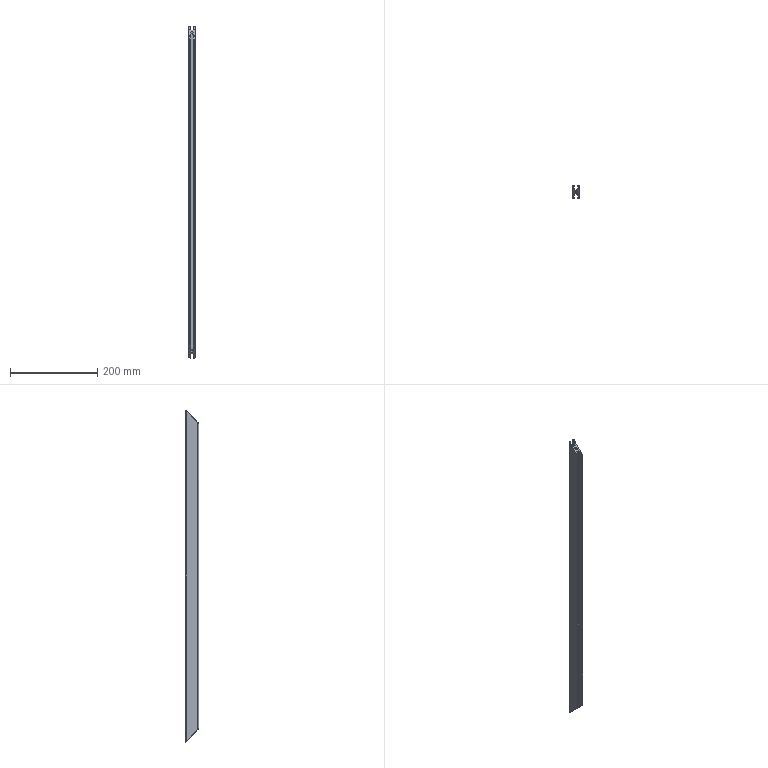Part | STEP file | OB1530-760 | 1 solid | 36 faces | box 15 x 30 x 760 mm | volume 178437 mm3 | plane 30 | cylinder 6 | commonest cylinder face diameters 3 x4 5 x2
STEP:
#1=CARTESIAN_POINT('',(2.5,0.,745.));
#2=VERTEX_POINT('',#1);
#3=CARTESIAN_POINT('',(-2.5,0.,745.));
#4=VERTEX_POINT('',#3);
#5=CARTESIAN_POINT('',(2.5,0.,745.));
#6=CARTESIAN_POINT('',(2.5,-5.,740.));
#7=CARTESIAN_POINT('',(-2.5,-5.,740.));
#8=CARTESIAN_POINT('',(-2.5,0.,745.));
#9=(BOUNDED_CURVE()B_SPLINE_CURVE(3,(#5,#6,#7,#8),.UNSPECIFIED.,.F.,.F.)B_SPLINE_CURVE_WITH_KNOTS((4,4),(4.712,7.854),.UNSPECIFIED.)CURVE()GEOMETRIC_REPRESENTATION_ITEM()RATIONAL_B_SPLINE_CURVE((1.,0.3333,0.3333,1.))REPRESENTATION_ITEM(''));
#10=EDGE_CURVE('',#2,#4,#9,.T.);
#11=ORIENTED_EDGE('',*,*,#10,.F.);
#12=CARTESIAN_POINT('',(2.5,0.,15.));
#13=VERTEX_POINT('',#12);
#14=CARTESIAN_POINT('',(2.5,0.,760.));
#15=DIRECTION('',(0.,0.,-1.));
#16=VECTOR('',#15,1000.);
#17=LINE('',#14,#16);
#18=EDGE_CURVE('',#2,#13,#17,.T.);
#19=ORIENTED_EDGE('',*,*,#18,.T.);
#20=CARTESIAN_POINT('',(-2.5,0.,15.));
#21=VERTEX_POINT('',#20);
#22=CARTESIAN_POINT('',(-2.5,0.,15.));
#23=CARTESIAN_POINT('',(-2.5,-5.,20.));
#24=CARTESIAN_POINT('',(2.5,-5.,20.));
#25=CARTESIAN_POINT('',(2.5,0.,15.));
#26=(BOUNDED_CURVE()B_SPLINE_CURVE(3,(#22,#23,#24,#25),.UNSPECIFIED.,.F.,.F.)B_SPLINE_CURVE_WITH_KNOTS((4,4),(1.571,4.712),.UNSPECIFIED.)CURVE()GEOMETRIC_REPRESENTATION_ITEM()RATIONAL_B_SPLINE_CURVE((1.,0.3333,0.3333,1.))REPRESENTATION_ITEM(''));
#27=EDGE_CURVE('',#21,#13,#26,.T.);
#28=ORIENTED_EDGE('',*,*,#27,.F.);
#29=CARTESIAN_POINT('',(-2.5,0.,760.));
#30=DIRECTION('',(0.,0.,-1.));
#31=VECTOR('',#30,1000.);
#32=LINE('',#29,#31);
#33=EDGE_CURVE('',#4,#21,#32,.T.);
#34=ORIENTED_EDGE('',*,*,#33,.F.);
#35=EDGE_LOOP('',(#11,#19,#28,#34));
#36=FACE_OUTER_BOUND('',#35,.T.);
#37=CARTESIAN_POINT('',(0.,0.,760.));
#38=DIRECTION('',(0.,0.,-1.));
#39=DIRECTION('',(-1.,0.,0.));
#40=AXIS2_PLACEMENT_3D('',#37,#38,#39);
#41=CYLINDRICAL_SURFACE('',#40,2.5);
#42=ADVANCED_FACE('',(#36),#41,.F.);
#43=CARTESIAN_POINT('',(6.,15.,760.));
#44=VERTEX_POINT('',#43);
#45=CARTESIAN_POINT('',(6.,15.,0.));
#46=VERTEX_POINT('',#45);
#47=CARTESIAN_POINT('',(6.,15.,760.));
#48=DIRECTION('',(0.,0.,-1.));
#49=VECTOR('',#48,1000.);
#50=LINE('',#47,#49);
#51=EDGE_CURVE('',#44,#46,#50,.T.);
#52=ORIENTED_EDGE('',*,*,#51,.F.);
#53=CARTESIAN_POINT('',(7.5,13.5,758.5));
#54=VERTEX_POINT('',#53);
#55=CARTESIAN_POINT('',(6.,15.,760.));
#56=CARTESIAN_POINT('',(6.879,15.,760.));
#57=CARTESIAN_POINT('',(7.5,14.379,759.379));
#58=CARTESIAN_POINT('',(7.5,13.5,758.5));
#59=(BOUNDED_CURVE()B_SPLINE_CURVE(3,(#55,#56,#57,#58),.UNSPECIFIED.,.F.,.T.)B_SPLINE_CURVE_WITH_KNOTS((4,4),(3.142,4.712),.UNSPECIFIED.)CURVE()GEOMETRIC_REPRESENTATION_ITEM()RATIONAL_B_SPLINE_CURVE((1.,0.8047,0.8047,1.))REPRESENTATION_ITEM(''));
#60=EDGE_CURVE('',#44,#54,#59,.T.);
#61=ORIENTED_EDGE('',*,*,#60,.T.);
#62=CARTESIAN_POINT('',(7.5,13.5,1.5));
#63=VERTEX_POINT('',#62);
#64=CARTESIAN_POINT('',(7.5,13.5,760.));
#65=DIRECTION('',(0.,0.,-1.));
#66=VECTOR('',#65,1000.);
#67=LINE('',#64,#66);
#68=EDGE_CURVE('',#54,#63,#67,.T.);
#69=ORIENTED_EDGE('',*,*,#68,.T.);
#70=CARTESIAN_POINT('',(7.5,13.5,1.5));
#71=CARTESIAN_POINT('',(7.5,14.379,0.6213));
#72=CARTESIAN_POINT('',(6.879,15.,0.));
#73=CARTESIAN_POINT('',(6.,15.,0.));
#74=(BOUNDED_CURVE()B_SPLINE_CURVE(3,(#70,#71,#72,#73),.UNSPECIFIED.,.F.,.F.)B_SPLINE_CURVE_WITH_KNOTS((4,4),(4.712,6.283),.UNSPECIFIED.)CURVE()GEOMETRIC_REPRESENTATION_ITEM()RATIONAL_B_SPLINE_CURVE((1.,0.8047,0.8047,1.))REPRESENTATION_ITEM(''));
#75=EDGE_CURVE('',#63,#46,#74,.T.);
#76=ORIENTED_EDGE('',*,*,#75,.T.);
#77=EDGE_LOOP('',(#52,#61,#69,#76));
#78=FACE_OUTER_BOUND('',#77,.T.);
#79=CARTESIAN_POINT('',(6.,13.5,760.));
#80=DIRECTION('',(0.,0.,-1.));
#81=DIRECTION('',(-1.,0.,0.));
#82=AXIS2_PLACEMENT_3D('',#79,#80,#81);
#83=CYLINDRICAL_SURFACE('',#82,1.5);
#84=ADVANCED_FACE('',(#78),#83,.T.);
#85=CARTESIAN_POINT('',(3.25,15.,0.));
#86=VERTEX_POINT('',#85);
#87=CARTESIAN_POINT('',(6.,15.,0.));
#88=DIRECTION('',(-1.,0.,0.));
#89=VECTOR('',#88,1000.);
#90=LINE('',#87,#89);
#91=EDGE_CURVE('',#46,#86,#90,.T.);
#92=ORIENTED_EDGE('',*,*,#91,.T.);
#93=CARTESIAN_POINT('',(3.25,15.,760.));
#94=VERTEX_POINT('',#93);
#95=CARTESIAN_POINT('',(3.25,15.,760.));
#96=DIRECTION('',(0.,0.,-1.));
#97=VECTOR('',#96,1000.);
#98=LINE('',#95,#97);
#99=EDGE_CURVE('',#94,#86,#98,.T.);
#100=ORIENTED_EDGE('',*,*,#99,.F.);
#101=CARTESIAN_POINT('',(6.,15.,760.));
#102=DIRECTION('',(-1.,0.,0.));
#103=VECTOR('',#102,1000.);
#104=LINE('',#101,#103);
#105=EDGE_CURVE('',#44,#94,#104,.T.);
#106=ORIENTED_EDGE('',*,*,#105,.F.);
#107=ORIENTED_EDGE('',*,*,#51,.T.);
#108=EDGE_LOOP('',(#92,#100,#106,#107));
#109=FACE_OUTER_BOUND('',#108,.T.);
#110=CARTESIAN_POINT('',(6.,15.,760.));
#111=DIRECTION('',(0.,-1.,0.));
#112=DIRECTION('',(0.,0.,-1.));
#113=AXIS2_PLACEMENT_3D('',#110,#111,#112);
#114=PLANE('',#113);
#115=ADVANCED_FACE('',(#109),#114,.F.);
#116=CARTESIAN_POINT('',(3.25,13.,758.));
#117=VERTEX_POINT('',#116);
#118=CARTESIAN_POINT('',(3.25,13.,2.));
#119=VERTEX_POINT('',#118);
#120=CARTESIAN_POINT('',(3.25,13.,760.));
#121=DIRECTION('',(0.,0.,-1.));
#122=VECTOR('',#121,1000.);
#123=LINE('',#120,#122);
#124=EDGE_CURVE('',#117,#119,#123,.T.);
#125=ORIENTED_EDGE('',*,*,#124,.F.);
#126=CARTESIAN_POINT('',(3.25,15.,760.));
#127=DIRECTION('',(0.,0.7071,0.7071));
#128=VECTOR('',#127,1000.);
#129=LINE('',#126,#128);
#130=EDGE_CURVE('',#117,#94,#129,.T.);
#131=ORIENTED_EDGE('',*,*,#130,.T.);
#132=ORIENTED_EDGE('',*,*,#99,.T.);
#133=CARTESIAN_POINT('',(3.25,-365.,380.));
#134=DIRECTION('',(0.,-0.7071,0.7071));
#135=VECTOR('',#134,1000.);
#136=LINE('',#133,#135);
#137=EDGE_CURVE('',#86,#119,#136,.T.);
#138=ORIENTED_EDGE('',*,*,#137,.T.);
#139=EDGE_LOOP('',(#125,#131,#132,#138));
#140=FACE_OUTER_BOUND('',#139,.T.);
#141=CARTESIAN_POINT('',(3.25,15.,760.));
#142=DIRECTION('',(1.,0.,0.));
#143=DIRECTION('',(0.,0.,-1.));
#144=AXIS2_PLACEMENT_3D('',#141,#142,#143);
#145=PLANE('',#144);
#146=ADVANCED_FACE('',(#140),#145,.F.);
#147=CARTESIAN_POINT('',(5.5,13.,758.));
#148=VERTEX_POINT('',#147);
#149=CARTESIAN_POINT('',(5.5,13.,2.));
#150=VERTEX_POINT('',#149);
#151=CARTESIAN_POINT('',(5.5,13.,760.));
#152=DIRECTION('',(0.,0.,-1.));
#153=VECTOR('',#152,1000.);
#154=LINE('',#151,#153);
#155=EDGE_CURVE('',#148,#150,#154,.T.);
#156=ORIENTED_EDGE('',*,*,#155,.F.);
#157=CARTESIAN_POINT('',(3.25,13.,758.));
#158=DIRECTION('',(-1.,0.,0.));
#159=VECTOR('',#158,1000.);
#160=LINE('',#157,#159);
#161=EDGE_CURVE('',#148,#117,#160,.T.);
#162=ORIENTED_EDGE('',*,*,#161,.T.);
#163=ORIENTED_EDGE('',*,*,#124,.T.);
#164=CARTESIAN_POINT('',(3.25,13.,2.));
#165=DIRECTION('',(1.,0.,0.));
#166=VECTOR('',#165,1000.);
#167=LINE('',#164,#166);
#168=EDGE_CURVE('',#119,#150,#167,.T.);
#169=ORIENTED_EDGE('',*,*,#168,.T.);
#170=EDGE_LOOP('',(#156,#162,#163,#169));
#171=FACE_OUTER_BOUND('',#170,.T.);
#172=CARTESIAN_POINT('',(3.25,13.,760.));
#173=DIRECTION('',(0.,1.,0.));
#174=DIRECTION('',(0.,0.,1.));
#175=AXIS2_PLACEMENT_3D('',#172,#173,#174);
#176=PLANE('',#175);
#177=ADVANCED_FACE('',(#171),#176,.F.);
#178=CARTESIAN_POINT('',(5.5,7.,752.));
#179=VERTEX_POINT('',#178);
#180=CARTESIAN_POINT('',(5.5,7.,8.));
#181=VERTEX_POINT('',#180);
#182=CARTESIAN_POINT('',(5.5,7.,760.));
#183=DIRECTION('',(0.,0.,-1.));
#184=VECTOR('',#183,1000.);
#185=LINE('',#182,#184);
#186=EDGE_CURVE('',#179,#181,#185,.T.);
#187=ORIENTED_EDGE('',*,*,#186,.F.);
#188=CARTESIAN_POINT('',(5.5,14.,759.));
#189=DIRECTION('',(0.,0.7071,0.7071));
#190=VECTOR('',#189,1000.);
#191=LINE('',#188,#190);
#192=EDGE_CURVE('',#179,#148,#191,.T.);
#193=ORIENTED_EDGE('',*,*,#192,.T.);
#194=ORIENTED_EDGE('',*,*,#155,.T.);
#195=CARTESIAN_POINT('',(5.5,-366.,381.));
#196=DIRECTION('',(0.,-0.7071,0.7071));
#197=VECTOR('',#196,1000.);
#198=LINE('',#195,#197);
#199=EDGE_CURVE('',#150,#181,#198,.T.);
#200=ORIENTED_EDGE('',*,*,#199,.T.);
#201=EDGE_LOOP('',(#187,#193,#194,#200));
#202=FACE_OUTER_BOUND('',#201,.T.);
#203=CARTESIAN_POINT('',(5.5,13.,760.));
#204=DIRECTION('',(1.,0.,0.));
#205=DIRECTION('',(0.,1.,0.));
#206=AXIS2_PLACEMENT_3D('',#203,#204,#205);
#207=PLANE('',#206);
#208=ADVANCED_FACE('',(#202),#207,.F.);
#209=CARTESIAN_POINT('',(3.25,7.,752.));
#210=VERTEX_POINT('',#209);
#211=CARTESIAN_POINT('',(3.25,7.,8.));
#212=VERTEX_POINT('',#211);
#213=CARTESIAN_POINT('',(3.25,7.,760.));
#214=DIRECTION('',(0.,0.,-1.));
#215=VECTOR('',#214,1000.);
#216=LINE('',#213,#215);
#217=EDGE_CURVE('',#210,#212,#216,.T.);
#218=ORIENTED_EDGE('',*,*,#217,.F.);
#219=CARTESIAN_POINT('',(5.5,7.,752.));
#220=DIRECTION('',(1.,0.,0.));
#221=VECTOR('',#220,1000.);
#222=LINE('',#219,#221);
#223=EDGE_CURVE('',#210,#179,#222,.T.);
#224=ORIENTED_EDGE('',*,*,#223,.T.);
#225=ORIENTED_EDGE('',*,*,#186,.T.);
#226=CARTESIAN_POINT('',(5.5,7.,8.));
#227=DIRECTION('',(-1.,0.,0.));
#228=VECTOR('',#227,1000.);
#229=LINE('',#226,#228);
#230=EDGE_CURVE('',#181,#212,#229,.T.);
#231=ORIENTED_EDGE('',*,*,#230,.T.);
#232=EDGE_LOOP('',(#218,#224,#225,#231));
#233=FACE_OUTER_BOUND('',#232,.T.);
#234=CARTESIAN_POINT('',(5.5,7.,760.));
#235=DIRECTION('',(0.,-1.,0.));
#236=DIRECTION('',(1.,0.,0.));
#237=AXIS2_PLACEMENT_3D('',#234,#235,#236);
#238=PLANE('',#237);
#239=ADVANCED_FACE('',(#233),#238,.F.);
#240=CARTESIAN_POINT('',(3.25,5.,750.));
#241=VERTEX_POINT('',#240);
#242=CARTESIAN_POINT('',(3.25,5.,10.));
#243=VERTEX_POINT('',#242);
#244=CARTESIAN_POINT('',(3.25,5.,760.));
#245=DIRECTION('',(0.,0.,-1.));
#246=VECTOR('',#245,1000.);
#247=LINE('',#244,#246);
#248=EDGE_CURVE('',#241,#243,#247,.T.);
#249=ORIENTED_EDGE('',*,*,#248,.F.);
#250=CARTESIAN_POINT('',(3.25,11.,756.));
#251=DIRECTION('',(0.,0.7071,0.7071));
#252=VECTOR('',#251,1000.);
#253=LINE('',#250,#252);
#254=EDGE_CURVE('',#241,#210,#253,.T.);
#255=ORIENTED_EDGE('',*,*,#254,.T.);
#256=ORIENTED_EDGE('',*,*,#217,.T.);
#257=CARTESIAN_POINT('',(3.25,-369.,384.));
#258=DIRECTION('',(0.,-0.7071,0.7071));
#259=VECTOR('',#258,1000.);
#260=LINE('',#257,#259);
#261=EDGE_CURVE('',#212,#243,#260,.T.);
#262=ORIENTED_EDGE('',*,*,#261,.T.);
#263=EDGE_LOOP('',(#249,#255,#256,#262));
#264=FACE_OUTER_BOUND('',#263,.T.);
#265=CARTESIAN_POINT('',(3.25,7.,760.));
#266=DIRECTION('',(1.,0.,0.));
#267=DIRECTION('',(0.,1.,0.));
#268=AXIS2_PLACEMENT_3D('',#265,#266,#267);
#269=PLANE('',#268);
#270=ADVANCED_FACE('',(#264),#269,.F.);
#271=CARTESIAN_POINT('',(-3.25,5.,750.));
#272=VERTEX_POINT('',#271);
#273=CARTESIAN_POINT('',(-3.25,5.,10.));
#274=VERTEX_POINT('',#273);
#275=CARTESIAN_POINT('',(-3.25,5.,760.));
#276=DIRECTION('',(0.,0.,-1.));
#277=VECTOR('',#276,1000.);
#278=LINE('',#275,#277);
#279=EDGE_CURVE('',#272,#274,#278,.T.);
#280=ORIENTED_EDGE('',*,*,#279,.F.);
#281=CARTESIAN_POINT('',(3.25,5.,750.));
#282=DIRECTION('',(1.,0.,0.));
#283=VECTOR('',#282,1000.);
#284=LINE('',#281,#283);
#285=EDGE_CURVE('',#272,#241,#284,.T.);
#286=ORIENTED_EDGE('',*,*,#285,.T.);
#287=ORIENTED_EDGE('',*,*,#248,.T.);
#288=CARTESIAN_POINT('',(3.25,5.,10.));
#289=DIRECTION('',(-1.,0.,0.));
#290=VECTOR('',#289,1000.);
#291=LINE('',#288,#290);
#292=EDGE_CURVE('',#243,#274,#291,.T.);
#293=ORIENTED_EDGE('',*,*,#292,.T.);
#294=EDGE_LOOP('',(#280,#286,#287,#293));
#295=FACE_OUTER_BOUND('',#294,.T.);
#296=CARTESIAN_POINT('',(3.25,5.,760.));
#297=DIRECTION('',(0.,-1.,0.));
#298=DIRECTION('',(0.,0.,-1.));
#299=AXIS2_PLACEMENT_3D('',#296,#297,#298);
#300=PLANE('',#299);
#301=ADVANCED_FACE('',(#295),#300,.F.);
#302=CARTESIAN_POINT('',(-3.25,7.,752.));
#303=VERTEX_POINT('',#302);
#304=CARTESIAN_POINT('',(-3.25,7.,8.));
#305=VERTEX_POINT('',#304);
#306=CARTESIAN_POINT('',(-3.25,7.,760.));
#307=DIRECTION('',(0.,0.,-1.));
#308=VECTOR('',#307,1000.);
#309=LINE('',#306,#308);
#310=EDGE_CURVE('',#303,#305,#309,.T.);
#311=ORIENTED_EDGE('',*,*,#310,.F.);
#312=CARTESIAN_POINT('',(-3.25,11.,756.));
#313=DIRECTION('',(0.,-0.7071,-0.7071));
#314=VECTOR('',#313,1000.);
#315=LINE('',#312,#314);
#316=EDGE_CURVE('',#303,#272,#315,.T.);
#317=ORIENTED_EDGE('',*,*,#316,.T.);
#318=ORIENTED_EDGE('',*,*,#279,.T.);
#319=CARTESIAN_POINT('',(-3.25,-369.,384.));
#320=DIRECTION('',(0.,0.7071,-0.7071));
#321=VECTOR('',#320,1000.);
#322=LINE('',#319,#321);
#323=EDGE_CURVE('',#274,#305,#322,.T.);
#324=ORIENTED_EDGE('',*,*,#323,.T.);
#325=EDGE_LOOP('',(#311,#317,#318,#324));
#326=FACE_OUTER_BOUND('',#325,.T.);
#327=CARTESIAN_POINT('',(-3.25,7.,760.));
#328=DIRECTION('',(-1.,0.,0.));
#329=DIRECTION('',(0.,-1.,0.));
#330=AXIS2_PLACEMENT_3D('',#327,#328,#329);
#331=PLANE('',#330);
#332=ADVANCED_FACE('',(#326),#331,.F.);
#333=CARTESIAN_POINT('',(-5.5,7.,752.));
#334=VERTEX_POINT('',#333);
#335=CARTESIAN_POINT('',(-5.5,7.,8.));
#336=VERTEX_POINT('',#335);
#337=CARTESIAN_POINT('',(-5.5,7.,760.));
#338=DIRECTION('',(0.,0.,-1.));
#339=VECTOR('',#338,1000.);
#340=LINE('',#337,#339);
#341=EDGE_CURVE('',#334,#336,#340,.T.);
#342=ORIENTED_EDGE('',*,*,#341,.F.);
#343=CARTESIAN_POINT('',(-5.5,7.,752.));
#344=DIRECTION('',(1.,0.,0.));
#345=VECTOR('',#344,1000.);
#346=LINE('',#343,#345);
#347=EDGE_CURVE('',#334,#303,#346,.T.);
#348=ORIENTED_EDGE('',*,*,#347,.T.);
#349=ORIENTED_EDGE('',*,*,#310,.T.);
#350=CARTESIAN_POINT('',(-5.5,7.,8.));
#351=DIRECTION('',(-1.,0.,0.));
#352=VECTOR('',#351,1000.);
#353=LINE('',#350,#352);
#354=EDGE_CURVE('',#305,#336,#353,.T.);
#355=ORIENTED_EDGE('',*,*,#354,.T.);
#356=EDGE_LOOP('',(#342,#348,#349,#355));
#357=FACE_OUTER_BOUND('',#356,.T.);
#358=CARTESIAN_POINT('',(-5.5,7.,760.));
#359=DIRECTION('',(0.,-1.,0.));
#360=DIRECTION('',(1.,0.,0.));
#361=AXIS2_PLACEMENT_3D('',#358,#359,#360);
#362=PLANE('',#361);
#363=ADVANCED_FACE('',(#357),#362,.F.);
#364=CARTESIAN_POINT('',(-5.5,13.,758.));
#365=VERTEX_POINT('',#364);
#366=CARTESIAN_POINT('',(-5.5,13.,2.));
#367=VERTEX_POINT('',#366);
#368=CARTESIAN_POINT('',(-5.5,13.,760.));
#369=DIRECTION('',(0.,0.,-1.));
#370=VECTOR('',#369,1000.);
#371=LINE('',#368,#370);
#372=EDGE_CURVE('',#365,#367,#371,.T.);
#373=ORIENTED_EDGE('',*,*,#372,.F.);
#374=CARTESIAN_POINT('',(-5.5,14.,759.));
#375=DIRECTION('',(0.,-0.7071,-0.7071));
#376=VECTOR('',#375,1000.);
#377=LINE('',#374,#376);
#378=EDGE_CURVE('',#365,#334,#377,.T.);
#379=ORIENTED_EDGE('',*,*,#378,.T.);
#380=ORIENTED_EDGE('',*,*,#341,.T.);
#381=CARTESIAN_POINT('',(-5.5,-366.,381.));
#382=DIRECTION('',(0.,0.7071,-0.7071));
#383=VECTOR('',#382,1000.);
#384=LINE('',#381,#383);
#385=EDGE_CURVE('',#336,#367,#384,.T.);
#386=ORIENTED_EDGE('',*,*,#385,.T.);
#387=EDGE_LOOP('',(#373,#379,#380,#386));
#388=FACE_OUTER_BOUND('',#387,.T.);
#389=CARTESIAN_POINT('',(-5.5,13.,760.));
#390=DIRECTION('',(-1.,0.,0.));
#391=DIRECTION('',(0.,-1.,0.));
#392=AXIS2_PLACEMENT_3D('',#389,#390,#391);
#393=PLANE('',#392);
#394=ADVANCED_FACE('',(#388),#393,.F.);
#395=CARTESIAN_POINT('',(-3.25,13.,758.));
#396=VERTEX_POINT('',#395);
#397=CARTESIAN_POINT('',(-3.25,13.,2.));
#398=VERTEX_POINT('',#397);
#399=CARTESIAN_POINT('',(-3.25,13.,760.));
#400=DIRECTION('',(0.,0.,-1.));
#401=VECTOR('',#400,1000.);
#402=LINE('',#399,#401);
#403=EDGE_CURVE('',#396,#398,#402,.T.);
#404=ORIENTED_EDGE('',*,*,#403,.F.);
#405=CARTESIAN_POINT('',(-3.25,13.,758.));
#406=DIRECTION('',(-1.,0.,0.));
#407=VECTOR('',#406,1000.);
#408=LINE('',#405,#407);
#409=EDGE_CURVE('',#396,#365,#408,.T.);
#410=ORIENTED_EDGE('',*,*,#409,.T.);
#411=ORIENTED_EDGE('',*,*,#372,.T.);
#412=CARTESIAN_POINT('',(-3.25,13.,2.));
#413=DIRECTION('',(1.,0.,0.));
#414=VECTOR('',#413,1000.);
#415=LINE('',#412,#414);
#416=EDGE_CURVE('',#367,#398,#415,.T.);
#417=ORIENTED_EDGE('',*,*,#416,.T.);
#418=EDGE_LOOP('',(#404,#410,#411,#417));
#419=FACE_OUTER_BOUND('',#418,.T.);
#420=CARTESIAN_POINT('',(-3.25,13.,760.));
#421=DIRECTION('',(0.,1.,0.));
#422=DIRECTION('',(0.,0.,1.));
#423=AXIS2_PLACEMENT_3D('',#420,#421,#422);
#424=PLANE('',#423);
#425=ADVANCED_FACE('',(#419),#424,.F.);
#426=CARTESIAN_POINT('',(-3.25,15.,760.));
#427=VERTEX_POINT('',#426);
#428=CARTESIAN_POINT('',(-3.25,15.,0.));
#429=VERTEX_POINT('',#428);
#430=CARTESIAN_POINT('',(-3.25,15.,760.));
#431=DIRECTION('',(0.,0.,-1.));
#432=VECTOR('',#431,1000.);
#433=LINE('',#430,#432);
#434=EDGE_CURVE('',#427,#429,#433,.T.);
#435=ORIENTED_EDGE('',*,*,#434,.F.);
#436=CARTESIAN_POINT('',(-3.25,15.,760.));
#437=DIRECTION('',(0.,-0.7071,-0.7071));
#438=VECTOR('',#437,1000.);
#439=LINE('',#436,#438);
#440=EDGE_CURVE('',#427,#396,#439,.T.);
#441=ORIENTED_EDGE('',*,*,#440,.T.);
#442=ORIENTED_EDGE('',*,*,#403,.T.);
#443=CARTESIAN_POINT('',(-3.25,-365.,380.));
#444=DIRECTION('',(0.,0.7071,-0.7071));
#445=VECTOR('',#444,1000.);
#446=LINE('',#443,#445);
#447=EDGE_CURVE('',#398,#429,#446,.T.);
#448=ORIENTED_EDGE('',*,*,#447,.T.);
#449=EDGE_LOOP('',(#435,#441,#442,#448));
#450=FACE_OUTER_BOUND('',#449,.T.);
#451=CARTESIAN_POINT('',(-3.25,15.,760.));
#452=DIRECTION('',(-1.,0.,0.));
#453=DIRECTION('',(0.,0.,1.));
#454=AXIS2_PLACEMENT_3D('',#451,#452,#453);
#455=PLANE('',#454);
#456=ADVANCED_FACE('',(#450),#455,.F.);
#457=CARTESIAN_POINT('',(-6.,15.,0.));
#458=VERTEX_POINT('',#457);
#459=CARTESIAN_POINT('',(-6.,15.,0.));
#460=DIRECTION('',(-1.,0.,0.));
#461=VECTOR('',#460,1000.);
#462=LINE('',#459,#461);
#463=EDGE_CURVE('',#429,#458,#462,.T.);
#464=ORIENTED_EDGE('',*,*,#463,.T.);
#465=CARTESIAN_POINT('',(-6.,15.,760.));
#466=VERTEX_POINT('',#465);
#467=CARTESIAN_POINT('',(-6.,15.,760.));
#468=DIRECTION('',(0.,0.,-1.));
#469=VECTOR('',#468,1000.);
#470=LINE('',#467,#469);
#471=EDGE_CURVE('',#466,#458,#470,.T.);
#472=ORIENTED_EDGE('',*,*,#471,.F.);
#473=CARTESIAN_POINT('',(-6.,15.,760.));
#474=DIRECTION('',(-1.,0.,0.));
#475=VECTOR('',#474,1000.);
#476=LINE('',#473,#475);
#477=EDGE_CURVE('',#427,#466,#476,.T.);
#478=ORIENTED_EDGE('',*,*,#477,.F.);
#479=ORIENTED_EDGE('',*,*,#434,.T.);
#480=EDGE_LOOP('',(#464,#472,#478,#479));
#481=FACE_OUTER_BOUND('',#480,.T.);
#482=CARTESIAN_POINT('',(-6.,15.,760.));
#483=DIRECTION('',(0.,-1.,0.));
#484=DIRECTION('',(0.,0.,-1.));
#485=AXIS2_PLACEMENT_3D('',#482,#483,#484);
#486=PLANE('',#485);
#487=ADVANCED_FACE('',(#481),#486,.F.);
#488=CARTESIAN_POINT('',(-7.5,13.5,758.5));
#489=VERTEX_POINT('',#488);
#490=CARTESIAN_POINT('',(-7.5,13.5,1.5));
#491=VERTEX_POINT('',#490);
#492=CARTESIAN_POINT('',(-7.5,13.5,760.));
#493=DIRECTION('',(0.,0.,-1.));
#494=VECTOR('',#493,1000.);
#495=LINE('',#492,#494);
#496=EDGE_CURVE('',#489,#491,#495,.T.);
#497=ORIENTED_EDGE('',*,*,#496,.F.);
#498=CARTESIAN_POINT('',(-7.5,13.5,758.5));
#499=CARTESIAN_POINT('',(-7.5,14.379,759.379));
#500=CARTESIAN_POINT('',(-6.879,15.,760.));
#501=CARTESIAN_POINT('',(-6.,15.,760.));
#502=(BOUNDED_CURVE()B_SPLINE_CURVE(3,(#498,#499,#500,#501),.UNSPECIFIED.,.F.,.T.)B_SPLINE_CURVE_WITH_KNOTS((4,4),(1.571,3.142),.UNSPECIFIED.)CURVE()GEOMETRIC_REPRESENTATION_ITEM()RATIONAL_B_SPLINE_CURVE((1.,0.8047,0.8047,1.))REPRESENTATION_ITEM(''));
#503=EDGE_CURVE('',#489,#466,#502,.T.);
#504=ORIENTED_EDGE('',*,*,#503,.T.);
#505=ORIENTED_EDGE('',*,*,#471,.T.);
#506=CARTESIAN_POINT('',(-6.,15.,0.));
#507=CARTESIAN_POINT('',(-6.879,15.,0.));
#508=CARTESIAN_POINT('',(-7.5,14.379,0.6213));
#509=CARTESIAN_POINT('',(-7.5,13.5,1.5));
#510=(BOUNDED_CURVE()B_SPLINE_CURVE(3,(#506,#507,#508,#509),.UNSPECIFIED.,.F.,.F.)B_SPLINE_CURVE_WITH_KNOTS((4,4),(0.,1.571),.UNSPECIFIED.)CURVE()GEOMETRIC_REPRESENTATION_ITEM()RATIONAL_B_SPLINE_CURVE((1.,0.8047,0.8047,1.))REPRESENTATION_ITEM(''));
#511=EDGE_CURVE('',#458,#491,#510,.T.);
#512=ORIENTED_EDGE('',*,*,#511,.T.);
#513=EDGE_LOOP('',(#497,#504,#505,#512));
#514=FACE_OUTER_BOUND('',#513,.T.);
#515=CARTESIAN_POINT('',(-6.,13.5,760.));
#516=DIRECTION('',(0.,0.,-1.));
#517=DIRECTION('',(-1.,0.,0.));
#518=AXIS2_PLACEMENT_3D('',#515,#516,#517);
#519=CYLINDRICAL_SURFACE('',#518,1.5);
#520=ADVANCED_FACE('',(#514),#519,.T.);
#521=CARTESIAN_POINT('',(-7.5,-13.5,731.5));
#522=VERTEX_POINT('',#521);
#523=CARTESIAN_POINT('',(-7.5,-13.5,28.5));
#524=VERTEX_POINT('',#523);
#525=CARTESIAN_POINT('',(-7.5,-13.5,760.));
#526=DIRECTION('',(0.,0.,-1.));
#527=VECTOR('',#526,1000.);
#528=LINE('',#525,#527);
#529=EDGE_CURVE('',#522,#524,#528,.T.);
#530=ORIENTED_EDGE('',*,*,#529,.F.);
#531=CARTESIAN_POINT('',(-7.5,-15.,730.));
#532=DIRECTION('',(0.,-0.7071,-0.7071));
#533=VECTOR('',#532,1000.);
#534=LINE('',#531,#533);
#535=EDGE_CURVE('',#489,#522,#534,.T.);
#536=ORIENTED_EDGE('',*,*,#535,.F.);
#537=ORIENTED_EDGE('',*,*,#496,.T.);
#538=CARTESIAN_POINT('',(-7.5,15.,0.));
#539=DIRECTION('',(0.,0.7071,-0.7071));
#540=VECTOR('',#539,1000.);
#541=LINE('',#538,#540);
#542=EDGE_CURVE('',#524,#491,#541,.T.);
#543=ORIENTED_EDGE('',*,*,#542,.F.);
#544=EDGE_LOOP('',(#530,#536,#537,#543));
#545=FACE_OUTER_BOUND('',#544,.T.);
#546=CARTESIAN_POINT('',(-7.5,-13.5,760.));
#547=DIRECTION('',(1.,0.,0.));
#548=DIRECTION('',(0.,0.,-1.));
#549=AXIS2_PLACEMENT_3D('',#546,#547,#548);
#550=PLANE('',#549);
#551=ADVANCED_FACE('',(#545),#550,.F.);
#552=CARTESIAN_POINT('',(-6.,-15.,730.));
#553=VERTEX_POINT('',#552);
#554=CARTESIAN_POINT('',(-6.,-15.,30.));
#555=VERTEX_POINT('',#554);
#556=CARTESIAN_POINT('',(-6.,-15.,760.));
#557=DIRECTION('',(0.,0.,-1.));
#558=VECTOR('',#557,1000.);
#559=LINE('',#556,#558);
#560=EDGE_CURVE('',#553,#555,#559,.T.);
#561=ORIENTED_EDGE('',*,*,#560,.F.);
#562=CARTESIAN_POINT('',(-6.,-15.,730.));
#563=CARTESIAN_POINT('',(-6.879,-15.,730.));
#564=CARTESIAN_POINT('',(-7.5,-14.379,730.621));
#565=CARTESIAN_POINT('',(-7.5,-13.5,731.5));
#566=(BOUNDED_CURVE()B_SPLINE_CURVE(3,(#562,#563,#564,#565),.UNSPECIFIED.,.F.,.F.)B_SPLINE_CURVE_WITH_KNOTS((4,4),(0.,1.571),.UNSPECIFIED.)CURVE()GEOMETRIC_REPRESENTATION_ITEM()RATIONAL_B_SPLINE_CURVE((1.,0.8047,0.8047,1.))REPRESENTATION_ITEM(''));
#567=EDGE_CURVE('',#553,#522,#566,.T.);
#568=ORIENTED_EDGE('',*,*,#567,.T.);
#569=ORIENTED_EDGE('',*,*,#529,.T.);
#570=CARTESIAN_POINT('',(-7.5,-13.5,28.5));
#571=CARTESIAN_POINT('',(-7.5,-14.379,29.379));
#572=CARTESIAN_POINT('',(-6.879,-15.,30.));
#573=CARTESIAN_POINT('',(-6.,-15.,30.));
#574=(BOUNDED_CURVE()B_SPLINE_CURVE(3,(#570,#571,#572,#573),.UNSPECIFIED.,.F.,.F.)B_SPLINE_CURVE_WITH_KNOTS((4,4),(1.571,3.142),.UNSPECIFIED.)CURVE()GEOMETRIC_REPRESENTATION_ITEM()RATIONAL_B_SPLINE_CURVE((1.,0.8047,0.8047,1.))REPRESENTATION_ITEM(''));
#575=EDGE_CURVE('',#524,#555,#574,.T.);
#576=ORIENTED_EDGE('',*,*,#575,.T.);
#577=EDGE_LOOP('',(#561,#568,#569,#576));
#578=FACE_OUTER_BOUND('',#577,.T.);
#579=CARTESIAN_POINT('',(-6.,-13.5,760.));
#580=DIRECTION('',(0.,0.,-1.));
#581=DIRECTION('',(-1.,0.,0.));
#582=AXIS2_PLACEMENT_3D('',#579,#580,#581);
#583=CYLINDRICAL_SURFACE('',#582,1.5);
#584=ADVANCED_FACE('',(#578),#583,.T.);
#585=CARTESIAN_POINT('',(-3.25,-15.,730.));
#586=VERTEX_POINT('',#585);
#587=CARTESIAN_POINT('',(-3.25,-15.,30.));
#588=VERTEX_POINT('',#587);
#589=CARTESIAN_POINT('',(-3.25,-15.,760.));
#590=DIRECTION('',(0.,0.,-1.));
#591=VECTOR('',#590,1000.);
#592=LINE('',#589,#591);
#593=EDGE_CURVE('',#586,#588,#592,.T.);
#594=ORIENTED_EDGE('',*,*,#593,.F.);
#595=CARTESIAN_POINT('',(7.5,-15.,730.));
#596=DIRECTION('',(-1.,0.,0.));
#597=VECTOR('',#596,1000.);
#598=LINE('',#595,#597);
#599=EDGE_CURVE('',#586,#553,#598,.T.);
#600=ORIENTED_EDGE('',*,*,#599,.T.);
#601=ORIENTED_EDGE('',*,*,#560,.T.);
#602=CARTESIAN_POINT('',(7.5,-15.,30.));
#603=DIRECTION('',(-1.,0.,0.));
#604=VECTOR('',#603,1000.);
#605=LINE('',#602,#604);
#606=EDGE_CURVE('',#588,#555,#605,.T.);
#607=ORIENTED_EDGE('',*,*,#606,.F.);
#608=EDGE_LOOP('',(#594,#600,#601,#607));
#609=FACE_OUTER_BOUND('',#608,.T.);
#610=CARTESIAN_POINT('',(-6.,-15.,760.));
#611=DIRECTION('',(0.,1.,0.));
#612=DIRECTION('',(0.,0.,1.));
#613=AXIS2_PLACEMENT_3D('',#610,#611,#612);
#614=PLANE('',#613);
#615=ADVANCED_FACE('',(#609),#614,.F.);
#616=CARTESIAN_POINT('',(-3.25,-13.,732.));
#617=VERTEX_POINT('',#616);
#618=CARTESIAN_POINT('',(-3.25,-13.,28.));
#619=VERTEX_POINT('',#618);
#620=CARTESIAN_POINT('',(-3.25,-13.,760.));
#621=DIRECTION('',(0.,0.,-1.));
#622=VECTOR('',#621,1000.);
#623=LINE('',#620,#622);
#624=EDGE_CURVE('',#617,#619,#623,.T.);
#625=ORIENTED_EDGE('',*,*,#624,.F.);
#626=CARTESIAN_POINT('',(-3.25,0.,745.));
#627=DIRECTION('',(0.,-0.7071,-0.7071));
#628=VECTOR('',#627,1000.);
#629=LINE('',#626,#628);
#630=EDGE_CURVE('',#617,#586,#629,.T.);
#631=ORIENTED_EDGE('',*,*,#630,.T.);
#632=ORIENTED_EDGE('',*,*,#593,.T.);
#633=CARTESIAN_POINT('',(-3.25,-380.,395.));
#634=DIRECTION('',(0.,0.7071,-0.7071));
#635=VECTOR('',#634,1000.);
#636=LINE('',#633,#635);
#637=EDGE_CURVE('',#588,#619,#636,.T.);
#638=ORIENTED_EDGE('',*,*,#637,.T.);
#639=EDGE_LOOP('',(#625,#631,#632,#638));
#640=FACE_OUTER_BOUND('',#639,.T.);
#641=CARTESIAN_POINT('',(-3.25,-15.,760.));
#642=DIRECTION('',(-1.,0.,0.));
#643=DIRECTION('',(0.,0.,1.));
#644=AXIS2_PLACEMENT_3D('',#641,#642,#643);
#645=PLANE('',#644);
#646=ADVANCED_FACE('',(#640),#645,.F.);
#647=CARTESIAN_POINT('',(-5.5,-13.,732.));
#648=VERTEX_POINT('',#647);
#649=CARTESIAN_POINT('',(-5.5,-13.,28.));
#650=VERTEX_POINT('',#649);
#651=CARTESIAN_POINT('',(-5.5,-13.,760.));
#652=DIRECTION('',(0.,0.,-1.));
#653=VECTOR('',#652,1000.);
#654=LINE('',#651,#653);
#655=EDGE_CURVE('',#648,#650,#654,.T.);
#656=ORIENTED_EDGE('',*,*,#655,.F.);
#657=CARTESIAN_POINT('',(-3.25,-13.,732.));
#658=DIRECTION('',(1.,0.,0.));
#659=VECTOR('',#658,1000.);
#660=LINE('',#657,#659);
#661=EDGE_CURVE('',#648,#617,#660,.T.);
#662=ORIENTED_EDGE('',*,*,#661,.T.);
#663=ORIENTED_EDGE('',*,*,#624,.T.);
#664=CARTESIAN_POINT('',(-3.25,-13.,28.));
#665=DIRECTION('',(-1.,0.,0.));
#666=VECTOR('',#665,1000.);
#667=LINE('',#664,#666);
#668=EDGE_CURVE('',#619,#650,#667,.T.);
#669=ORIENTED_EDGE('',*,*,#668,.T.);
#670=EDGE_LOOP('',(#656,#662,#663,#669));
#671=FACE_OUTER_BOUND('',#670,.T.);
#672=CARTESIAN_POINT('',(-3.25,-13.,760.));
#673=DIRECTION('',(0.,-1.,0.));
#674=DIRECTION('',(0.,0.,-1.));
#675=AXIS2_PLACEMENT_3D('',#672,#673,#674);
#676=PLANE('',#675);
#677=ADVANCED_FACE('',(#671),#676,.F.);
#678=CARTESIAN_POINT('',(-5.5,-7.,738.));
#679=VERTEX_POINT('',#678);
#680=CARTESIAN_POINT('',(-5.5,-7.,22.));
#681=VERTEX_POINT('',#680);
#682=CARTESIAN_POINT('',(-5.5,-7.,760.));
#683=DIRECTION('',(0.,0.,-1.));
#684=VECTOR('',#683,1000.);
#685=LINE('',#682,#684);
#686=EDGE_CURVE('',#679,#681,#685,.T.);
#687=ORIENTED_EDGE('',*,*,#686,.F.);
#688=CARTESIAN_POINT('',(-5.5,1.,746.));
#689=DIRECTION('',(0.,-0.7071,-0.7071));
#690=VECTOR('',#689,1000.);
#691=LINE('',#688,#690);
#692=EDGE_CURVE('',#679,#648,#691,.T.);
#693=ORIENTED_EDGE('',*,*,#692,.T.);
#694=ORIENTED_EDGE('',*,*,#655,.T.);
#695=CARTESIAN_POINT('',(-5.5,-379.,394.));
#696=DIRECTION('',(0.,0.7071,-0.7071));
#697=VECTOR('',#696,1000.);
#698=LINE('',#695,#697);
#699=EDGE_CURVE('',#650,#681,#698,.T.);
#700=ORIENTED_EDGE('',*,*,#699,.T.);
#701=EDGE_LOOP('',(#687,#693,#694,#700));
#702=FACE_OUTER_BOUND('',#701,.T.);
#703=CARTESIAN_POINT('',(-5.5,-13.,760.));
#704=DIRECTION('',(-1.,0.,0.));
#705=DIRECTION('',(0.,-1.,0.));
#706=AXIS2_PLACEMENT_3D('',#703,#704,#705);
#707=PLANE('',#706);
#708=ADVANCED_FACE('',(#702),#707,.F.);
#709=CARTESIAN_POINT('',(-3.25,-7.,738.));
#710=VERTEX_POINT('',#709);
#711=CARTESIAN_POINT('',(-3.25,-7.,22.));
#712=VERTEX_POINT('',#711);
#713=CARTESIAN_POINT('',(-3.25,-7.,760.));
#714=DIRECTION('',(0.,0.,-1.));
#715=VECTOR('',#714,1000.);
#716=LINE('',#713,#715);
#717=EDGE_CURVE('',#710,#712,#716,.T.);
#718=ORIENTED_EDGE('',*,*,#717,.F.);
#719=CARTESIAN_POINT('',(-5.5,-7.,738.));
#720=DIRECTION('',(-1.,0.,0.));
#721=VECTOR('',#720,1000.);
#722=LINE('',#719,#721);
#723=EDGE_CURVE('',#710,#679,#722,.T.);
#724=ORIENTED_EDGE('',*,*,#723,.T.);
#725=ORIENTED_EDGE('',*,*,#686,.T.);
#726=CARTESIAN_POINT('',(-5.5,-7.,22.));
#727=DIRECTION('',(1.,0.,0.));
#728=VECTOR('',#727,1000.);
#729=LINE('',#726,#728);
#730=EDGE_CURVE('',#681,#712,#729,.T.);
#731=ORIENTED_EDGE('',*,*,#730,.T.);
#732=EDGE_LOOP('',(#718,#724,#725,#731));
#733=FACE_OUTER_BOUND('',#732,.T.);
#734=CARTESIAN_POINT('',(-5.5,-7.,760.));
#735=DIRECTION('',(0.,1.,0.));
#736=DIRECTION('',(-1.,0.,0.));
#737=AXIS2_PLACEMENT_3D('',#734,#735,#736);
#738=PLANE('',#737);
#739=ADVANCED_FACE('',(#733),#738,.F.);
#740=CARTESIAN_POINT('',(-3.25,-5.,740.));
#741=VERTEX_POINT('',#740);
#742=CARTESIAN_POINT('',(-3.25,-5.,20.));
#743=VERTEX_POINT('',#742);
#744=CARTESIAN_POINT('',(-3.25,-5.,760.));
#745=DIRECTION('',(0.,0.,-1.));
#746=VECTOR('',#745,1000.);
#747=LINE('',#744,#746);
#748=EDGE_CURVE('',#741,#743,#747,.T.);
#749=ORIENTED_EDGE('',*,*,#748,.F.);
#750=CARTESIAN_POINT('',(-3.25,4.,749.));
#751=DIRECTION('',(0.,-0.7071,-0.7071));
#752=VECTOR('',#751,1000.);
#753=LINE('',#750,#752);
#754=EDGE_CURVE('',#741,#710,#753,.T.);
#755=ORIENTED_EDGE('',*,*,#754,.T.);
#756=ORIENTED_EDGE('',*,*,#717,.T.);
#757=CARTESIAN_POINT('',(-3.25,-376.,391.));
#758=DIRECTION('',(0.,0.7071,-0.7071));
#759=VECTOR('',#758,1000.);
#760=LINE('',#757,#759);
#761=EDGE_CURVE('',#712,#743,#760,.T.);
#762=ORIENTED_EDGE('',*,*,#761,.T.);
#763=EDGE_LOOP('',(#749,#755,#756,#762));
#764=FACE_OUTER_BOUND('',#763,.T.);
#765=CARTESIAN_POINT('',(-3.25,-7.,760.));
#766=DIRECTION('',(-1.,0.,0.));
#767=DIRECTION('',(0.,-1.,0.));
#768=AXIS2_PLACEMENT_3D('',#765,#766,#767);
#769=PLANE('',#768);
#770=ADVANCED_FACE('',(#764),#769,.F.);
#771=CARTESIAN_POINT('',(3.25,-5.,740.));
#772=VERTEX_POINT('',#771);
#773=CARTESIAN_POINT('',(3.25,-5.,20.));
#774=VERTEX_POINT('',#773);
#775=CARTESIAN_POINT('',(3.25,-5.,760.));
#776=DIRECTION('',(0.,0.,-1.));
#777=VECTOR('',#776,1000.);
#778=LINE('',#775,#777);
#779=EDGE_CURVE('',#772,#774,#778,.T.);
#780=ORIENTED_EDGE('',*,*,#779,.F.);
#781=CARTESIAN_POINT('',(3.25,-5.,740.));
#782=DIRECTION('',(-1.,0.,0.));
#783=VECTOR('',#782,1000.);
#784=LINE('',#781,#783);
#785=EDGE_CURVE('',#772,#741,#784,.T.);
#786=ORIENTED_EDGE('',*,*,#785,.T.);
#787=ORIENTED_EDGE('',*,*,#748,.T.);
#788=CARTESIAN_POINT('',(3.25,-5.,20.));
#789=DIRECTION('',(1.,0.,0.));
#790=VECTOR('',#789,1000.);
#791=LINE('',#788,#790);
#792=EDGE_CURVE('',#743,#774,#791,.T.);
#793=ORIENTED_EDGE('',*,*,#792,.T.);
#794=EDGE_LOOP('',(#780,#786,#787,#793));
#795=FACE_OUTER_BOUND('',#794,.T.);
#796=CARTESIAN_POINT('',(3.25,-5.,760.));
#797=DIRECTION('',(0.,1.,0.));
#798=DIRECTION('',(0.,0.,1.));
#799=AXIS2_PLACEMENT_3D('',#796,#797,#798);
#800=PLANE('',#799);
#801=ADVANCED_FACE('',(#795),#800,.F.);
#802=CARTESIAN_POINT('',(3.25,-7.,738.));
#803=VERTEX_POINT('',#802);
#804=CARTESIAN_POINT('',(3.25,-7.,22.));
#805=VERTEX_POINT('',#804);
#806=CARTESIAN_POINT('',(3.25,-7.,760.));
#807=DIRECTION('',(0.,0.,-1.));
#808=VECTOR('',#807,1000.);
#809=LINE('',#806,#808);
#810=EDGE_CURVE('',#803,#805,#809,.T.);
#811=ORIENTED_EDGE('',*,*,#810,.F.);
#812=CARTESIAN_POINT('',(3.25,4.,749.));
#813=DIRECTION('',(0.,0.7071,0.7071));
#814=VECTOR('',#813,1000.);
#815=LINE('',#812,#814);
#816=EDGE_CURVE('',#803,#772,#815,.T.);
#817=ORIENTED_EDGE('',*,*,#816,.T.);
#818=ORIENTED_EDGE('',*,*,#779,.T.);
#819=CARTESIAN_POINT('',(3.25,-376.,391.));
#820=DIRECTION('',(0.,-0.7071,0.7071));
#821=VECTOR('',#820,1000.);
#822=LINE('',#819,#821);
#823=EDGE_CURVE('',#774,#805,#822,.T.);
#824=ORIENTED_EDGE('',*,*,#823,.T.);
#825=EDGE_LOOP('',(#811,#817,#818,#824));
#826=FACE_OUTER_BOUND('',#825,.T.);
#827=CARTESIAN_POINT('',(3.25,-7.,760.));
#828=DIRECTION('',(1.,0.,0.));
#829=DIRECTION('',(0.,1.,0.));
#830=AXIS2_PLACEMENT_3D('',#827,#828,#829);
#831=PLANE('',#830);
#832=ADVANCED_FACE('',(#826),#831,.F.);
#833=CARTESIAN_POINT('',(5.5,-7.,738.));
#834=VERTEX_POINT('',#833);
#835=CARTESIAN_POINT('',(5.5,-7.,22.));
#836=VERTEX_POINT('',#835);
#837=CARTESIAN_POINT('',(5.5,-7.,760.));
#838=DIRECTION('',(0.,0.,-1.));
#839=VECTOR('',#838,1000.);
#840=LINE('',#837,#839);
#841=EDGE_CURVE('',#834,#836,#840,.T.);
#842=ORIENTED_EDGE('',*,*,#841,.F.);
#843=CARTESIAN_POINT('',(5.5,-7.,738.));
#844=DIRECTION('',(-1.,0.,0.));
#845=VECTOR('',#844,1000.);
#846=LINE('',#843,#845);
#847=EDGE_CURVE('',#834,#803,#846,.T.);
#848=ORIENTED_EDGE('',*,*,#847,.T.);
#849=ORIENTED_EDGE('',*,*,#810,.T.);
#850=CARTESIAN_POINT('',(5.5,-7.,22.));
#851=DIRECTION('',(1.,0.,0.));
#852=VECTOR('',#851,1000.);
#853=LINE('',#850,#852);
#854=EDGE_CURVE('',#805,#836,#853,.T.);
#855=ORIENTED_EDGE('',*,*,#854,.T.);
#856=EDGE_LOOP('',(#842,#848,#849,#855));
#857=FACE_OUTER_BOUND('',#856,.T.);
#858=CARTESIAN_POINT('',(5.5,-7.,760.));
#859=DIRECTION('',(0.,1.,0.));
#860=DIRECTION('',(-1.,0.,0.));
#861=AXIS2_PLACEMENT_3D('',#858,#859,#860);
#862=PLANE('',#861);
#863=ADVANCED_FACE('',(#857),#862,.F.);
#864=CARTESIAN_POINT('',(5.5,-13.,732.));
#865=VERTEX_POINT('',#864);
#866=CARTESIAN_POINT('',(5.5,-13.,28.));
#867=VERTEX_POINT('',#866);
#868=CARTESIAN_POINT('',(5.5,-13.,760.));
#869=DIRECTION('',(0.,0.,-1.));
#870=VECTOR('',#869,1000.);
#871=LINE('',#868,#870);
#872=EDGE_CURVE('',#865,#867,#871,.T.);
#873=ORIENTED_EDGE('',*,*,#872,.F.);
#874=CARTESIAN_POINT('',(5.5,1.,746.));
#875=DIRECTION('',(0.,0.7071,0.7071));
#876=VECTOR('',#875,1000.);
#877=LINE('',#874,#876);
#878=EDGE_CURVE('',#865,#834,#877,.T.);
#879=ORIENTED_EDGE('',*,*,#878,.T.);
#880=ORIENTED_EDGE('',*,*,#841,.T.);
#881=CARTESIAN_POINT('',(5.5,-379.,394.));
#882=DIRECTION('',(0.,-0.7071,0.7071));
#883=VECTOR('',#882,1000.);
#884=LINE('',#881,#883);
#885=EDGE_CURVE('',#836,#867,#884,.T.);
#886=ORIENTED_EDGE('',*,*,#885,.T.);
#887=EDGE_LOOP('',(#873,#879,#880,#886));
#888=FACE_OUTER_BOUND('',#887,.T.);
#889=CARTESIAN_POINT('',(5.5,-13.,760.));
#890=DIRECTION('',(1.,0.,0.));
#891=DIRECTION('',(0.,1.,0.));
#892=AXIS2_PLACEMENT_3D('',#889,#890,#891);
#893=PLANE('',#892);
#894=ADVANCED_FACE('',(#888),#893,.F.);
#895=CARTESIAN_POINT('',(3.25,-13.,732.));
#896=VERTEX_POINT('',#895);
#897=CARTESIAN_POINT('',(3.25,-13.,28.));
#898=VERTEX_POINT('',#897);
#899=CARTESIAN_POINT('',(3.25,-13.,760.));
#900=DIRECTION('',(0.,0.,-1.));
#901=VECTOR('',#900,1000.);
#902=LINE('',#899,#901);
#903=EDGE_CURVE('',#896,#898,#902,.T.);
#904=ORIENTED_EDGE('',*,*,#903,.F.);
#905=CARTESIAN_POINT('',(3.25,-13.,732.));
#906=DIRECTION('',(1.,0.,0.));
#907=VECTOR('',#906,1000.);
#908=LINE('',#905,#907);
#909=EDGE_CURVE('',#896,#865,#908,.T.);
#910=ORIENTED_EDGE('',*,*,#909,.T.);
#911=ORIENTED_EDGE('',*,*,#872,.T.);
#912=CARTESIAN_POINT('',(3.25,-13.,28.));
#913=DIRECTION('',(-1.,0.,0.));
#914=VECTOR('',#913,1000.);
#915=LINE('',#912,#914);
#916=EDGE_CURVE('',#867,#898,#915,.T.);
#917=ORIENTED_EDGE('',*,*,#916,.T.);
#918=EDGE_LOOP('',(#904,#910,#911,#917));
#919=FACE_OUTER_BOUND('',#918,.T.);
#920=CARTESIAN_POINT('',(3.25,-13.,760.));
#921=DIRECTION('',(0.,-1.,0.));
#922=DIRECTION('',(0.,0.,-1.));
#923=AXIS2_PLACEMENT_3D('',#920,#921,#922);
#924=PLANE('',#923);
#925=ADVANCED_FACE('',(#919),#924,.F.);
#926=CARTESIAN_POINT('',(3.25,-15.,730.));
#927=VERTEX_POINT('',#926);
#928=CARTESIAN_POINT('',(3.25,-15.,30.));
#929=VERTEX_POINT('',#928);
#930=CARTESIAN_POINT('',(3.25,-15.,760.));
#931=DIRECTION('',(0.,0.,-1.));
#932=VECTOR('',#931,1000.);
#933=LINE('',#930,#932);
#934=EDGE_CURVE('',#927,#929,#933,.T.);
#935=ORIENTED_EDGE('',*,*,#934,.F.);
#936=CARTESIAN_POINT('',(3.25,0.,745.));
#937=DIRECTION('',(0.,0.7071,0.7071));
#938=VECTOR('',#937,1000.);
#939=LINE('',#936,#938);
#940=EDGE_CURVE('',#927,#896,#939,.T.);
#941=ORIENTED_EDGE('',*,*,#940,.T.);
#942=ORIENTED_EDGE('',*,*,#903,.T.);
#943=CARTESIAN_POINT('',(3.25,-380.,395.));
#944=DIRECTION('',(0.,-0.7071,0.7071));
#945=VECTOR('',#944,1000.);
#946=LINE('',#943,#945);
#947=EDGE_CURVE('',#898,#929,#946,.T.);
#948=ORIENTED_EDGE('',*,*,#947,.T.);
#949=EDGE_LOOP('',(#935,#941,#942,#948));
#950=FACE_OUTER_BOUND('',#949,.T.);
#951=CARTESIAN_POINT('',(3.25,-15.,760.));
#952=DIRECTION('',(1.,0.,0.));
#953=DIRECTION('',(0.,0.,-1.));
#954=AXIS2_PLACEMENT_3D('',#951,#952,#953);
#955=PLANE('',#954);
#956=ADVANCED_FACE('',(#950),#955,.F.);
#957=CARTESIAN_POINT('',(6.,-15.,730.));
#958=VERTEX_POINT('',#957);
#959=CARTESIAN_POINT('',(6.,-15.,30.));
#960=VERTEX_POINT('',#959);
#961=CARTESIAN_POINT('',(6.,-15.,760.));
#962=DIRECTION('',(0.,0.,-1.));
#963=VECTOR('',#962,1000.);
#964=LINE('',#961,#963);
#965=EDGE_CURVE('',#958,#960,#964,.T.);
#966=ORIENTED_EDGE('',*,*,#965,.F.);
#967=CARTESIAN_POINT('',(7.5,-15.,730.));
#968=DIRECTION('',(-1.,0.,0.));
#969=VECTOR('',#968,1000.);
#970=LINE('',#967,#969);
#971=EDGE_CURVE('',#958,#927,#970,.T.);
#972=ORIENTED_EDGE('',*,*,#971,.T.);
#973=ORIENTED_EDGE('',*,*,#934,.T.);
#974=CARTESIAN_POINT('',(7.5,-15.,30.));
#975=DIRECTION('',(-1.,0.,0.));
#976=VECTOR('',#975,1000.);
#977=LINE('',#974,#976);
#978=EDGE_CURVE('',#960,#929,#977,.T.);
#979=ORIENTED_EDGE('',*,*,#978,.F.);
#980=EDGE_LOOP('',(#966,#972,#973,#979));
#981=FACE_OUTER_BOUND('',#980,.T.);
#982=CARTESIAN_POINT('',(6.,-15.,760.));
#983=DIRECTION('',(0.,1.,0.));
#984=DIRECTION('',(0.,0.,1.));
#985=AXIS2_PLACEMENT_3D('',#982,#983,#984);
#986=PLANE('',#985);
#987=ADVANCED_FACE('',(#981),#986,.F.);
#988=CARTESIAN_POINT('',(7.5,-13.5,731.5));
#989=VERTEX_POINT('',#988);
#990=CARTESIAN_POINT('',(7.5,-13.5,28.5));
#991=VERTEX_POINT('',#990);
#992=CARTESIAN_POINT('',(7.5,-13.5,760.));
#993=DIRECTION('',(0.,0.,-1.));
#994=VECTOR('',#993,1000.);
#995=LINE('',#992,#994);
#996=EDGE_CURVE('',#989,#991,#995,.T.);
#997=ORIENTED_EDGE('',*,*,#996,.F.);
#998=CARTESIAN_POINT('',(7.5,-13.5,731.5));
#999=CARTESIAN_POINT('',(7.5,-14.379,730.621));
#1000=CARTESIAN_POINT('',(6.879,-15.,730.));
#1001=CARTESIAN_POINT('',(6.,-15.,730.));
#1002=(BOUNDED_CURVE()B_SPLINE_CURVE(3,(#998,#999,#1000,#1001),.UNSPECIFIED.,.F.,.F.)B_SPLINE_CURVE_WITH_KNOTS((4,4),(4.712,6.283),.UNSPECIFIED.)CURVE()GEOMETRIC_REPRESENTATION_ITEM()RATIONAL_B_SPLINE_CURVE((1.,0.8047,0.8047,1.))REPRESENTATION_ITEM(''));
#1003=EDGE_CURVE('',#989,#958,#1002,.T.);
#1004=ORIENTED_EDGE('',*,*,#1003,.T.);
#1005=ORIENTED_EDGE('',*,*,#965,.T.);
#1006=CARTESIAN_POINT('',(6.,-15.,30.));
#1007=CARTESIAN_POINT('',(6.879,-15.,30.));
#1008=CARTESIAN_POINT('',(7.5,-14.379,29.379));
#1009=CARTESIAN_POINT('',(7.5,-13.5,28.5));
#1010=(BOUNDED_CURVE()B_SPLINE_CURVE(3,(#1006,#1007,#1008,#1009),.UNSPECIFIED.,.F.,.T.)B_SPLINE_CURVE_WITH_KNOTS((4,4),(3.142,4.712),.UNSPECIFIED.)CURVE()GEOMETRIC_REPRESENTATION_ITEM()RATIONAL_B_SPLINE_CURVE((1.,0.8047,0.8047,1.))REPRESENTATION_ITEM(''));
#1011=EDGE_CURVE('',#960,#991,#1010,.T.);
#1012=ORIENTED_EDGE('',*,*,#1011,.T.);
#1013=EDGE_LOOP('',(#997,#1004,#1005,#1012));
#1014=FACE_OUTER_BOUND('',#1013,.T.);
#1015=CARTESIAN_POINT('',(6.,-13.5,760.));
#1016=DIRECTION('',(0.,0.,-1.));
#1017=DIRECTION('',(-1.,0.,0.));
#1018=AXIS2_PLACEMENT_3D('',#1015,#1016,#1017);
#1019=CYLINDRICAL_SURFACE('',#1018,1.5);
#1020=ADVANCED_FACE('',(#1014),#1019,.T.);
#1021=ORIENTED_EDGE('',*,*,#68,.F.);
#1022=CARTESIAN_POINT('',(7.5,-15.,730.));
#1023=DIRECTION('',(0.,-0.7071,-0.7071));
#1024=VECTOR('',#1023,1000.);
#1025=LINE('',#1022,#1024);
#1026=EDGE_CURVE('',#54,#989,#1025,.T.);
#1027=ORIENTED_EDGE('',*,*,#1026,.T.);
#1028=ORIENTED_EDGE('',*,*,#996,.T.);
#1029=CARTESIAN_POINT('',(7.5,15.,0.));
#1030=DIRECTION('',(0.,0.7071,-0.7071));
#1031=VECTOR('',#1030,1000.);
#1032=LINE('',#1029,#1031);
#1033=EDGE_CURVE('',#991,#63,#1032,.T.);
#1034=ORIENTED_EDGE('',*,*,#1033,.T.);
#1035=EDGE_LOOP('',(#1021,#1027,#1028,#1034));
#1036=FACE_OUTER_BOUND('',#1035,.T.);
#1037=CARTESIAN_POINT('',(7.5,-13.5,760.));
#1038=DIRECTION('',(-1.,0.,0.));
#1039=DIRECTION('',(0.,0.,1.));
#1040=AXIS2_PLACEMENT_3D('',#1037,#1038,#1039);
#1041=PLANE('',#1040);
#1042=ADVANCED_FACE('',(#1036),#1041,.F.);
#1043=ORIENTED_EDGE('',*,*,#18,.F.);
#1044=CARTESIAN_POINT('',(-2.5,0.,745.));
#1045=CARTESIAN_POINT('',(-2.5,5.,750.));
#1046=CARTESIAN_POINT('',(2.5,5.,750.));
#1047=CARTESIAN_POINT('',(2.5,0.,745.));
#1048=(BOUNDED_CURVE()B_SPLINE_CURVE(3,(#1044,#1045,#1046,#1047),.UNSPECIFIED.,.F.,.T.)B_SPLINE_CURVE_WITH_KNOTS((4,4),(1.571,4.712),.UNSPECIFIED.)CURVE()GEOMETRIC_REPRESENTATION_ITEM()RATIONAL_B_SPLINE_CURVE((1.,0.3333,0.3333,1.))REPRESENTATION_ITEM(''));
#1049=EDGE_CURVE('',#4,#2,#1048,.T.);
#1050=ORIENTED_EDGE('',*,*,#1049,.F.);
#1051=ORIENTED_EDGE('',*,*,#33,.T.);
#1052=CARTESIAN_POINT('',(2.5,0.,15.));
#1053=CARTESIAN_POINT('',(2.5,5.,10.));
#1054=CARTESIAN_POINT('',(-2.5,5.,10.));
#1055=CARTESIAN_POINT('',(-2.5,0.,15.));
#1056=(BOUNDED_CURVE()B_SPLINE_CURVE(3,(#1052,#1053,#1054,#1055),.UNSPECIFIED.,.F.,.F.)B_SPLINE_CURVE_WITH_KNOTS((4,4),(4.712,7.854),.UNSPECIFIED.)CURVE()GEOMETRIC_REPRESENTATION_ITEM()RATIONAL_B_SPLINE_CURVE((1.,0.3333,0.3333,1.))REPRESENTATION_ITEM(''));
#1057=EDGE_CURVE('',#13,#21,#1056,.T.);
#1058=ORIENTED_EDGE('',*,*,#1057,.F.);
#1059=EDGE_LOOP('',(#1043,#1050,#1051,#1058));
#1060=FACE_OUTER_BOUND('',#1059,.T.);
#1061=CARTESIAN_POINT('',(0.,0.,760.));
#1062=DIRECTION('',(0.,0.,-1.));
#1063=DIRECTION('',(-1.,0.,0.));
#1064=AXIS2_PLACEMENT_3D('',#1061,#1062,#1063);
#1065=CYLINDRICAL_SURFACE('',#1064,2.5);
#1066=ADVANCED_FACE('',(#1060),#1065,.F.);
#1067=ORIENTED_EDGE('',*,*,#27,.T.);
#1068=ORIENTED_EDGE('',*,*,#1057,.T.);
#1069=EDGE_LOOP('',(#1067,#1068));
#1070=FACE_BOUND('',#1069,.T.);
#1071=ORIENTED_EDGE('',*,*,#1033,.F.);
#1072=ORIENTED_EDGE('',*,*,#1011,.F.);
#1073=ORIENTED_EDGE('',*,*,#978,.T.);
#1074=ORIENTED_EDGE('',*,*,#947,.F.);
#1075=ORIENTED_EDGE('',*,*,#916,.F.);
#1076=ORIENTED_EDGE('',*,*,#885,.F.);
#1077=ORIENTED_EDGE('',*,*,#854,.F.);
#1078=ORIENTED_EDGE('',*,*,#823,.F.);
#1079=ORIENTED_EDGE('',*,*,#792,.F.);
#1080=ORIENTED_EDGE('',*,*,#761,.F.);
#1081=ORIENTED_EDGE('',*,*,#730,.F.);
#1082=ORIENTED_EDGE('',*,*,#699,.F.);
#1083=ORIENTED_EDGE('',*,*,#668,.F.);
#1084=ORIENTED_EDGE('',*,*,#637,.F.);
#1085=ORIENTED_EDGE('',*,*,#606,.T.);
#1086=ORIENTED_EDGE('',*,*,#575,.F.);
#1087=ORIENTED_EDGE('',*,*,#542,.T.);
#1088=ORIENTED_EDGE('',*,*,#511,.F.);
#1089=ORIENTED_EDGE('',*,*,#463,.F.);
#1090=ORIENTED_EDGE('',*,*,#447,.F.);
#1091=ORIENTED_EDGE('',*,*,#416,.F.);
#1092=ORIENTED_EDGE('',*,*,#385,.F.);
#1093=ORIENTED_EDGE('',*,*,#354,.F.);
#1094=ORIENTED_EDGE('',*,*,#323,.F.);
#1095=ORIENTED_EDGE('',*,*,#292,.F.);
#1096=ORIENTED_EDGE('',*,*,#261,.F.);
#1097=ORIENTED_EDGE('',*,*,#230,.F.);
#1098=ORIENTED_EDGE('',*,*,#199,.F.);
#1099=ORIENTED_EDGE('',*,*,#168,.F.);
#1100=ORIENTED_EDGE('',*,*,#137,.F.);
#1101=ORIENTED_EDGE('',*,*,#91,.F.);
#1102=ORIENTED_EDGE('',*,*,#75,.F.);
#1103=EDGE_LOOP('',(#1071,#1072,#1073,#1074,#1075,#1076,#1077,#1078,#1079,#1080,#1081,#1082,#1083,#1084,#1085,#1086,#1087,#1088,#1089,#1090,#1091,#1092,#1093,#1094,#1095,#1096,#1097,#1098,#1099,#1100,#1101,#1102));
#1104=FACE_OUTER_BOUND('',#1103,.T.);
#1105=CARTESIAN_POINT('',(7.5,15.,0.));
#1106=DIRECTION('',(0.,0.7071,0.7071));
#1107=DIRECTION('',(0.,-0.7071,0.7071));
#1108=AXIS2_PLACEMENT_3D('',#1105,#1106,#1107);
#1109=PLANE('',#1108);
#1110=ADVANCED_FACE('',(#1070,#1104),#1109,.F.);
#1111=ORIENTED_EDGE('',*,*,#1049,.T.);
#1112=ORIENTED_EDGE('',*,*,#10,.T.);
#1113=EDGE_LOOP('',(#1111,#1112));
#1114=FACE_BOUND('',#1113,.T.);
#1115=ORIENTED_EDGE('',*,*,#105,.T.);
#1116=ORIENTED_EDGE('',*,*,#130,.F.);
#1117=ORIENTED_EDGE('',*,*,#161,.F.);
#1118=ORIENTED_EDGE('',*,*,#192,.F.);
#1119=ORIENTED_EDGE('',*,*,#223,.F.);
#1120=ORIENTED_EDGE('',*,*,#254,.F.);
#1121=ORIENTED_EDGE('',*,*,#285,.F.);
#1122=ORIENTED_EDGE('',*,*,#316,.F.);
#1123=ORIENTED_EDGE('',*,*,#347,.F.);
#1124=ORIENTED_EDGE('',*,*,#378,.F.);
#1125=ORIENTED_EDGE('',*,*,#409,.F.);
#1126=ORIENTED_EDGE('',*,*,#440,.F.);
#1127=ORIENTED_EDGE('',*,*,#477,.T.);
#1128=ORIENTED_EDGE('',*,*,#503,.F.);
#1129=ORIENTED_EDGE('',*,*,#535,.T.);
#1130=ORIENTED_EDGE('',*,*,#567,.F.);
#1131=ORIENTED_EDGE('',*,*,#599,.F.);
#1132=ORIENTED_EDGE('',*,*,#630,.F.);
#1133=ORIENTED_EDGE('',*,*,#661,.F.);
#1134=ORIENTED_EDGE('',*,*,#692,.F.);
#1135=ORIENTED_EDGE('',*,*,#723,.F.);
#1136=ORIENTED_EDGE('',*,*,#754,.F.);
#1137=ORIENTED_EDGE('',*,*,#785,.F.);
#1138=ORIENTED_EDGE('',*,*,#816,.F.);
#1139=ORIENTED_EDGE('',*,*,#847,.F.);
#1140=ORIENTED_EDGE('',*,*,#878,.F.);
#1141=ORIENTED_EDGE('',*,*,#909,.F.);
#1142=ORIENTED_EDGE('',*,*,#940,.F.);
#1143=ORIENTED_EDGE('',*,*,#971,.F.);
#1144=ORIENTED_EDGE('',*,*,#1003,.F.);
#1145=ORIENTED_EDGE('',*,*,#1026,.F.);
#1146=ORIENTED_EDGE('',*,*,#60,.F.);
#1147=EDGE_LOOP('',(#1115,#1116,#1117,#1118,#1119,#1120,#1121,#1122,#1123,#1124,#1125,#1126,#1127,#1128,#1129,#1130,#1131,#1132,#1133,#1134,#1135,#1136,#1137,#1138,#1139,#1140,#1141,#1142,#1143,#1144,#1145,#1146));
#1148=FACE_OUTER_BOUND('',#1147,.T.);
#1149=CARTESIAN_POINT('',(7.5,-15.,730.));
#1150=DIRECTION('',(0.,0.7071,-0.7071));
#1151=DIRECTION('',(0.,0.7071,0.7071));
#1152=AXIS2_PLACEMENT_3D('',#1149,#1150,#1151);
#1153=PLANE('',#1152);
#1154=ADVANCED_FACE('',(#1114,#1148),#1153,.F.);
#1155=CLOSED_SHELL('',(#42,#84,#115,#146,#177,#208,#239,#270,#301,#332,#363,#394,#425,#456,#487,#520,#551,#584,#615,#646,#677,#708,#739,#770,#801,#832,#863,#894,#925,#956,#987,#1020,#1042,#1066,#1110,#1154));
#1156=MANIFOLD_SOLID_BREP('',#1155);
#1157=CARTESIAN_POINT('',(0.,0.,0.));
#1158=DIRECTION('',(0.,0.,1.));
#1159=DIRECTION('',(1.,0.,0.));
#1160=AXIS2_PLACEMENT_3D('',#1157,#1158,#1159);
#1161=(LENGTH_UNIT()NAMED_UNIT(*)SI_UNIT(.MILLI.,.METRE.));
#1162=UNCERTAINTY_MEASURE_WITH_UNIT(LENGTH_MEASURE(0.00001),#1161,'','');
#1163=(NAMED_UNIT(*)PLANE_ANGLE_UNIT()SI_UNIT($,.RADIAN.));
#1164=(NAMED_UNIT(*)SI_UNIT($,.STERADIAN.)SOLID_ANGLE_UNIT());
#1165=(GEOMETRIC_REPRESENTATION_CONTEXT(3)GLOBAL_UNCERTAINTY_ASSIGNED_CONTEXT((#1162))GLOBAL_UNIT_ASSIGNED_CONTEXT((#1161,#1163,#1164))REPRESENTATION_CONTEXT('',''));
#1166=ADVANCED_BREP_SHAPE_REPRESENTATION('',(#1156,#1160),#1165);